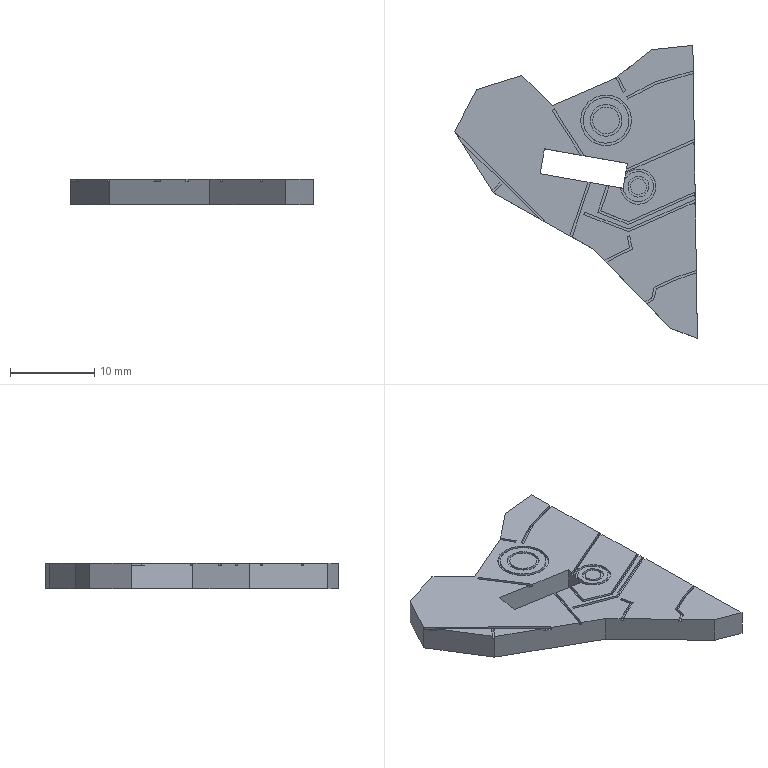Part | SolidWorks | features BaseBody 1 | 1 solid | 140 faces | box 28.805 x 34.776 x 3 mm | volume 1576 mm3 | plane 90 | spline 50